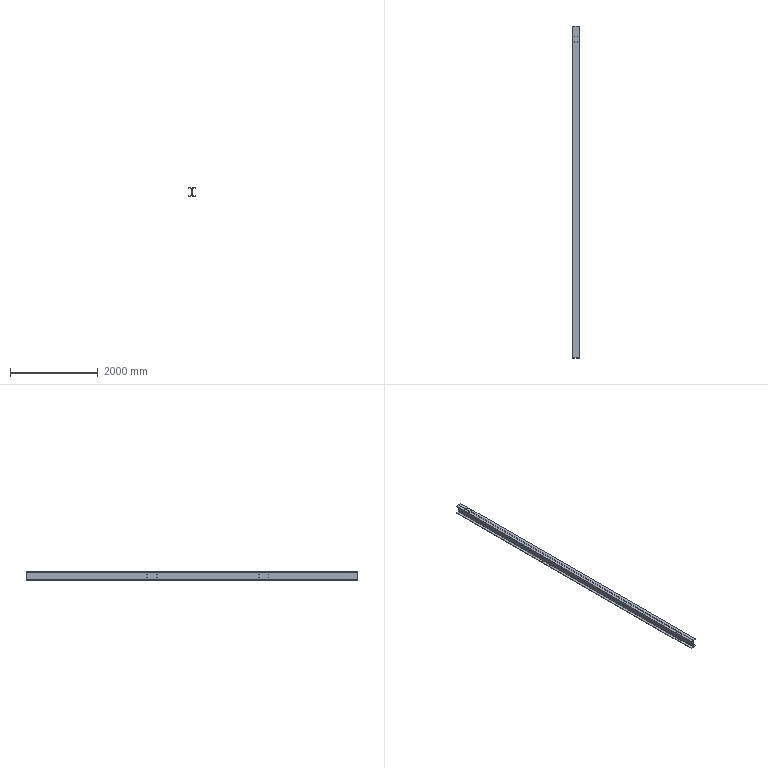Part | STEP file | Powder bin column 5 body_Default<As Machined> | 1 solid | 50 faces | box 150 x 7578 x 194 mm | volume 28858083 mm3 | cylinder 36 | plane 14 | commonest cylinder face diameters 15 x32 16 x4